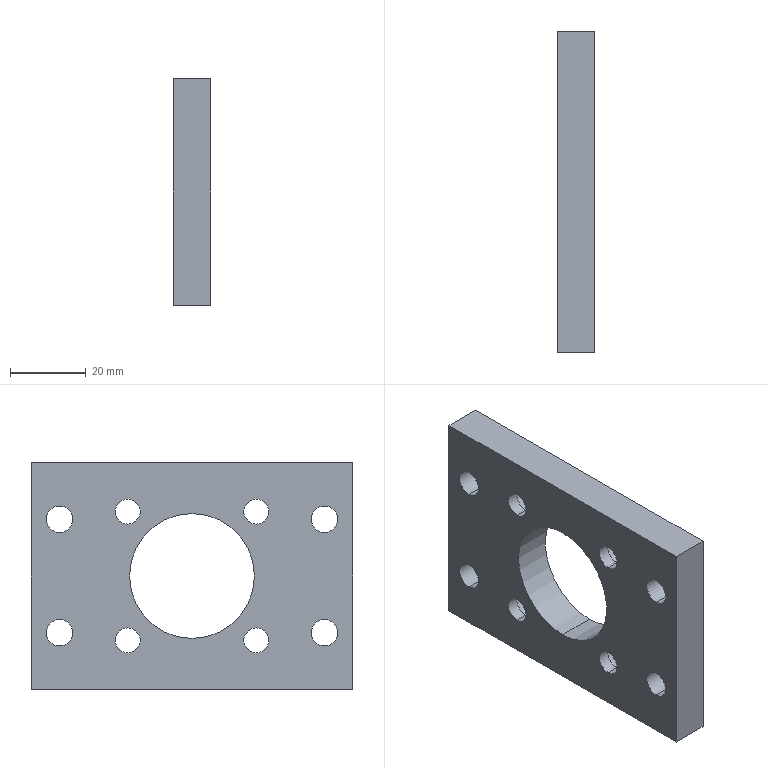Part | SolidWorks | features HoleWzd 2, Extrusion 1, ICE 1 | 1 solid | 36 faces | box 10 x 85 x 60 mm | volume 37885 mm3 | cylinder 26 | plane 10 | commonest cylinder face diameters 6.6 x8 7 x8 11 x8 33 x2
STEP:
#1=CARTESIAN_POINT('',(10.,0.,-16.5));
#2=VERTEX_POINT('',#1);
#3=CARTESIAN_POINT('',(10.,0.,16.5));
#4=VERTEX_POINT('',#3);
#5=CARTESIAN_POINT('',(10.,0.,0.));
#6=DIRECTION('',(-1.,0.,0.));
#7=DIRECTION('',(0.,0.,1.));
#8=AXIS2_PLACEMENT_3D('',#5,#6,#7);
#9=CIRCLE('',#8,16.5);
#10=EDGE_CURVE('',#2,#4,#9,.T.);
#11=ORIENTED_EDGE('',*,*,#10,.F.);
#12=CARTESIAN_POINT('',(0.,0.,-16.5));
#13=VERTEX_POINT('',#12);
#14=CARTESIAN_POINT('',(10.,0.,-16.5));
#15=DIRECTION('',(-1.,0.,0.));
#16=VECTOR('',#15,1000.);
#17=LINE('',#14,#16);
#18=EDGE_CURVE('',#2,#13,#17,.T.);
#19=ORIENTED_EDGE('',*,*,#18,.T.);
#20=CARTESIAN_POINT('',(0.,0.,16.5));
#21=VERTEX_POINT('',#20);
#22=CARTESIAN_POINT('',(0.,0.,0.));
#23=DIRECTION('',(-1.,0.,0.));
#24=DIRECTION('',(0.,0.,1.));
#25=AXIS2_PLACEMENT_3D('',#22,#23,#24);
#26=CIRCLE('',#25,16.5);
#27=EDGE_CURVE('',#13,#21,#26,.T.);
#28=ORIENTED_EDGE('',*,*,#27,.T.);
#29=CARTESIAN_POINT('',(10.,0.,16.5));
#30=DIRECTION('',(-1.,0.,0.));
#31=VECTOR('',#30,1000.);
#32=LINE('',#29,#31);
#33=EDGE_CURVE('',#4,#21,#32,.T.);
#34=ORIENTED_EDGE('',*,*,#33,.F.);
#35=EDGE_LOOP('',(#11,#19,#28,#34));
#36=FACE_OUTER_BOUND('',#35,.T.);
#37=CARTESIAN_POINT('',(10.,0.,0.));
#38=DIRECTION('',(-1.,0.,0.));
#39=DIRECTION('',(0.,0.,1.));
#40=AXIS2_PLACEMENT_3D('',#37,#38,#39);
#41=CYLINDRICAL_SURFACE('',#40,16.5);
#42=ADVANCED_FACE('',(#36),#41,.F.);
#43=CARTESIAN_POINT('',(10.,35.,-18.5));
#44=VERTEX_POINT('',#43);
#45=CARTESIAN_POINT('',(10.,35.,-11.5));
#46=VERTEX_POINT('',#45);
#47=CARTESIAN_POINT('',(10.,35.,-15.));
#48=DIRECTION('',(-1.,0.,0.));
#49=DIRECTION('',(0.,0.,1.));
#50=AXIS2_PLACEMENT_3D('',#47,#48,#49);
#51=CIRCLE('',#50,3.5);
#52=EDGE_CURVE('',#44,#46,#51,.T.);
#53=ORIENTED_EDGE('',*,*,#52,.F.);
#54=CARTESIAN_POINT('',(0.,35.,-18.5));
#55=VERTEX_POINT('',#54);
#56=CARTESIAN_POINT('',(0.,35.,-18.5));
#57=DIRECTION('',(-1.,0.,0.));
#58=VECTOR('',#57,1000.);
#59=LINE('',#56,#58);
#60=EDGE_CURVE('',#44,#55,#59,.T.);
#61=ORIENTED_EDGE('',*,*,#60,.T.);
#62=CARTESIAN_POINT('',(0.,35.,-11.5));
#63=VERTEX_POINT('',#62);
#64=CARTESIAN_POINT('',(0.,35.,-15.));
#65=DIRECTION('',(-1.,0.,0.));
#66=DIRECTION('',(0.,0.,1.));
#67=AXIS2_PLACEMENT_3D('',#64,#65,#66);
#68=CIRCLE('',#67,3.5);
#69=EDGE_CURVE('',#55,#63,#68,.T.);
#70=ORIENTED_EDGE('',*,*,#69,.T.);
#71=CARTESIAN_POINT('',(0.,35.,-11.5));
#72=DIRECTION('',(-1.,0.,0.));
#73=VECTOR('',#72,1000.);
#74=LINE('',#71,#73);
#75=EDGE_CURVE('',#46,#63,#74,.T.);
#76=ORIENTED_EDGE('',*,*,#75,.F.);
#77=EDGE_LOOP('',(#53,#61,#70,#76));
#78=FACE_OUTER_BOUND('',#77,.T.);
#79=CARTESIAN_POINT('',(0.,35.,-15.));
#80=DIRECTION('',(-1.,0.,0.));
#81=DIRECTION('',(0.,0.,1.));
#82=AXIS2_PLACEMENT_3D('',#79,#80,#81);
#83=CYLINDRICAL_SURFACE('',#82,3.5);
#84=ADVANCED_FACE('',(#78),#83,.F.);
#85=CARTESIAN_POINT('',(10.,35.,11.5));
#86=VERTEX_POINT('',#85);
#87=CARTESIAN_POINT('',(10.,35.,18.5));
#88=VERTEX_POINT('',#87);
#89=CARTESIAN_POINT('',(10.,35.,15.));
#90=DIRECTION('',(-1.,0.,0.));
#91=DIRECTION('',(0.,0.,1.));
#92=AXIS2_PLACEMENT_3D('',#89,#90,#91);
#93=CIRCLE('',#92,3.5);
#94=EDGE_CURVE('',#86,#88,#93,.T.);
#95=ORIENTED_EDGE('',*,*,#94,.F.);
#96=CARTESIAN_POINT('',(0.,35.,11.5));
#97=VERTEX_POINT('',#96);
#98=CARTESIAN_POINT('',(0.,35.,11.5));
#99=DIRECTION('',(-1.,0.,0.));
#100=VECTOR('',#99,1000.);
#101=LINE('',#98,#100);
#102=EDGE_CURVE('',#86,#97,#101,.T.);
#103=ORIENTED_EDGE('',*,*,#102,.T.);
#104=CARTESIAN_POINT('',(0.,35.,18.5));
#105=VERTEX_POINT('',#104);
#106=CARTESIAN_POINT('',(0.,35.,15.));
#107=DIRECTION('',(-1.,0.,0.));
#108=DIRECTION('',(0.,0.,1.));
#109=AXIS2_PLACEMENT_3D('',#106,#107,#108);
#110=CIRCLE('',#109,3.5);
#111=EDGE_CURVE('',#97,#105,#110,.T.);
#112=ORIENTED_EDGE('',*,*,#111,.T.);
#113=CARTESIAN_POINT('',(0.,35.,18.5));
#114=DIRECTION('',(-1.,0.,0.));
#115=VECTOR('',#114,1000.);
#116=LINE('',#113,#115);
#117=EDGE_CURVE('',#88,#105,#116,.T.);
#118=ORIENTED_EDGE('',*,*,#117,.F.);
#119=EDGE_LOOP('',(#95,#103,#112,#118));
#120=FACE_OUTER_BOUND('',#119,.T.);
#121=CARTESIAN_POINT('',(0.,35.,15.));
#122=DIRECTION('',(-1.,0.,0.));
#123=DIRECTION('',(0.,0.,1.));
#124=AXIS2_PLACEMENT_3D('',#121,#122,#123);
#125=CYLINDRICAL_SURFACE('',#124,3.5);
#126=ADVANCED_FACE('',(#120),#125,.F.);
#127=CARTESIAN_POINT('',(10.,-35.,-18.5));
#128=VERTEX_POINT('',#127);
#129=CARTESIAN_POINT('',(10.,-35.,-11.5));
#130=VERTEX_POINT('',#129);
#131=CARTESIAN_POINT('',(10.,-35.,-15.));
#132=DIRECTION('',(-1.,0.,0.));
#133=DIRECTION('',(0.,0.,1.));
#134=AXIS2_PLACEMENT_3D('',#131,#132,#133);
#135=CIRCLE('',#134,3.5);
#136=EDGE_CURVE('',#128,#130,#135,.T.);
#137=ORIENTED_EDGE('',*,*,#136,.F.);
#138=CARTESIAN_POINT('',(0.,-35.,-18.5));
#139=VERTEX_POINT('',#138);
#140=CARTESIAN_POINT('',(0.,-35.,-18.5));
#141=DIRECTION('',(-1.,0.,0.));
#142=VECTOR('',#141,1000.);
#143=LINE('',#140,#142);
#144=EDGE_CURVE('',#128,#139,#143,.T.);
#145=ORIENTED_EDGE('',*,*,#144,.T.);
#146=CARTESIAN_POINT('',(0.,-35.,-11.5));
#147=VERTEX_POINT('',#146);
#148=CARTESIAN_POINT('',(0.,-35.,-15.));
#149=DIRECTION('',(-1.,0.,0.));
#150=DIRECTION('',(0.,0.,1.));
#151=AXIS2_PLACEMENT_3D('',#148,#149,#150);
#152=CIRCLE('',#151,3.5);
#153=EDGE_CURVE('',#139,#147,#152,.T.);
#154=ORIENTED_EDGE('',*,*,#153,.T.);
#155=CARTESIAN_POINT('',(0.,-35.,-11.5));
#156=DIRECTION('',(-1.,0.,0.));
#157=VECTOR('',#156,1000.);
#158=LINE('',#155,#157);
#159=EDGE_CURVE('',#130,#147,#158,.T.);
#160=ORIENTED_EDGE('',*,*,#159,.F.);
#161=EDGE_LOOP('',(#137,#145,#154,#160));
#162=FACE_OUTER_BOUND('',#161,.T.);
#163=CARTESIAN_POINT('',(0.,-35.,-15.));
#164=DIRECTION('',(-1.,0.,0.));
#165=DIRECTION('',(0.,0.,1.));
#166=AXIS2_PLACEMENT_3D('',#163,#164,#165);
#167=CYLINDRICAL_SURFACE('',#166,3.5);
#168=ADVANCED_FACE('',(#162),#167,.F.);
#169=CARTESIAN_POINT('',(10.,-35.,11.5));
#170=VERTEX_POINT('',#169);
#171=CARTESIAN_POINT('',(10.,-35.,18.5));
#172=VERTEX_POINT('',#171);
#173=CARTESIAN_POINT('',(10.,-35.,15.));
#174=DIRECTION('',(-1.,0.,0.));
#175=DIRECTION('',(0.,0.,1.));
#176=AXIS2_PLACEMENT_3D('',#173,#174,#175);
#177=CIRCLE('',#176,3.5);
#178=EDGE_CURVE('',#170,#172,#177,.T.);
#179=ORIENTED_EDGE('',*,*,#178,.F.);
#180=CARTESIAN_POINT('',(0.,-35.,11.5));
#181=VERTEX_POINT('',#180);
#182=CARTESIAN_POINT('',(0.,-35.,11.5));
#183=DIRECTION('',(-1.,0.,0.));
#184=VECTOR('',#183,1000.);
#185=LINE('',#182,#184);
#186=EDGE_CURVE('',#170,#181,#185,.T.);
#187=ORIENTED_EDGE('',*,*,#186,.T.);
#188=CARTESIAN_POINT('',(0.,-35.,18.5));
#189=VERTEX_POINT('',#188);
#190=CARTESIAN_POINT('',(0.,-35.,15.));
#191=DIRECTION('',(-1.,0.,0.));
#192=DIRECTION('',(0.,0.,1.));
#193=AXIS2_PLACEMENT_3D('',#190,#191,#192);
#194=CIRCLE('',#193,3.5);
#195=EDGE_CURVE('',#181,#189,#194,.T.);
#196=ORIENTED_EDGE('',*,*,#195,.T.);
#197=CARTESIAN_POINT('',(0.,-35.,18.5));
#198=DIRECTION('',(-1.,0.,0.));
#199=VECTOR('',#198,1000.);
#200=LINE('',#197,#199);
#201=EDGE_CURVE('',#172,#189,#200,.T.);
#202=ORIENTED_EDGE('',*,*,#201,.F.);
#203=EDGE_LOOP('',(#179,#187,#196,#202));
#204=FACE_OUTER_BOUND('',#203,.T.);
#205=CARTESIAN_POINT('',(0.,-35.,15.));
#206=DIRECTION('',(-1.,0.,0.));
#207=DIRECTION('',(0.,0.,1.));
#208=AXIS2_PLACEMENT_3D('',#205,#206,#207);
#209=CYLINDRICAL_SURFACE('',#208,3.5);
#210=ADVANCED_FACE('',(#204),#209,.F.);
#211=CARTESIAN_POINT('',(3.2,17.,22.5));
#212=VERTEX_POINT('',#211);
#213=CARTESIAN_POINT('',(3.2,17.,11.5));
#214=VERTEX_POINT('',#213);
#215=CARTESIAN_POINT('',(3.2,17.,17.));
#216=DIRECTION('',(1.,0.,0.));
#217=DIRECTION('',(0.,0.,-1.));
#218=AXIS2_PLACEMENT_3D('',#215,#216,#217);
#219=CIRCLE('',#218,5.5);
#220=EDGE_CURVE('',#212,#214,#219,.T.);
#221=ORIENTED_EDGE('',*,*,#220,.F.);
#222=CARTESIAN_POINT('',(10.,17.,22.5));
#223=VERTEX_POINT('',#222);
#224=CARTESIAN_POINT('',(10.,17.,22.5));
#225=DIRECTION('',(1.,0.,0.));
#226=VECTOR('',#225,1000.);
#227=LINE('',#224,#226);
#228=EDGE_CURVE('',#212,#223,#227,.T.);
#229=ORIENTED_EDGE('',*,*,#228,.T.);
#230=CARTESIAN_POINT('',(10.,17.,11.5));
#231=VERTEX_POINT('',#230);
#232=CARTESIAN_POINT('',(10.,17.,17.));
#233=DIRECTION('',(1.,0.,0.));
#234=DIRECTION('',(0.,0.,-1.));
#235=AXIS2_PLACEMENT_3D('',#232,#233,#234);
#236=CIRCLE('',#235,5.5);
#237=EDGE_CURVE('',#223,#231,#236,.T.);
#238=ORIENTED_EDGE('',*,*,#237,.T.);
#239=CARTESIAN_POINT('',(10.,17.,11.5));
#240=DIRECTION('',(1.,0.,0.));
#241=VECTOR('',#240,1000.);
#242=LINE('',#239,#241);
#243=EDGE_CURVE('',#214,#231,#242,.T.);
#244=ORIENTED_EDGE('',*,*,#243,.F.);
#245=EDGE_LOOP('',(#221,#229,#238,#244));
#246=FACE_OUTER_BOUND('',#245,.T.);
#247=CARTESIAN_POINT('',(10.,17.,17.));
#248=DIRECTION('',(1.,0.,0.));
#249=DIRECTION('',(0.,0.,-1.));
#250=AXIS2_PLACEMENT_3D('',#247,#248,#249);
#251=CYLINDRICAL_SURFACE('',#250,5.5);
#252=ADVANCED_FACE('',(#246),#251,.F.);
#253=CARTESIAN_POINT('',(0.,17.,20.3));
#254=VERTEX_POINT('',#253);
#255=CARTESIAN_POINT('',(0.,17.,13.7));
#256=VERTEX_POINT('',#255);
#257=CARTESIAN_POINT('',(0.,17.,17.));
#258=DIRECTION('',(1.,0.,0.));
#259=DIRECTION('',(0.,0.,-1.));
#260=AXIS2_PLACEMENT_3D('',#257,#258,#259);
#261=CIRCLE('',#260,3.3);
#262=EDGE_CURVE('',#254,#256,#261,.T.);
#263=ORIENTED_EDGE('',*,*,#262,.F.);
#264=CARTESIAN_POINT('',(3.2,17.,20.3));
#265=VERTEX_POINT('',#264);
#266=CARTESIAN_POINT('',(10.,17.,20.3));
#267=DIRECTION('',(1.,0.,0.));
#268=VECTOR('',#267,1000.);
#269=LINE('',#266,#268);
#270=EDGE_CURVE('',#254,#265,#269,.T.);
#271=ORIENTED_EDGE('',*,*,#270,.T.);
#272=CARTESIAN_POINT('',(3.2,17.,13.7));
#273=VERTEX_POINT('',#272);
#274=CARTESIAN_POINT('',(3.2,17.,17.));
#275=DIRECTION('',(1.,0.,0.));
#276=DIRECTION('',(0.,0.,-1.));
#277=AXIS2_PLACEMENT_3D('',#274,#275,#276);
#278=CIRCLE('',#277,3.3);
#279=EDGE_CURVE('',#265,#273,#278,.T.);
#280=ORIENTED_EDGE('',*,*,#279,.T.);
#281=CARTESIAN_POINT('',(10.,17.,13.7));
#282=DIRECTION('',(1.,0.,0.));
#283=VECTOR('',#282,1000.);
#284=LINE('',#281,#283);
#285=EDGE_CURVE('',#256,#273,#284,.T.);
#286=ORIENTED_EDGE('',*,*,#285,.F.);
#287=EDGE_LOOP('',(#263,#271,#280,#286));
#288=FACE_OUTER_BOUND('',#287,.T.);
#289=CARTESIAN_POINT('',(10.,17.,17.));
#290=DIRECTION('',(1.,0.,0.));
#291=DIRECTION('',(0.,0.,-1.));
#292=AXIS2_PLACEMENT_3D('',#289,#290,#291);
#293=CYLINDRICAL_SURFACE('',#292,3.3);
#294=ADVANCED_FACE('',(#288),#293,.F.);
#295=CARTESIAN_POINT('',(3.2,17.,-11.5));
#296=VERTEX_POINT('',#295);
#297=CARTESIAN_POINT('',(3.2,17.,-22.5));
#298=VERTEX_POINT('',#297);
#299=CARTESIAN_POINT('',(3.2,17.,-17.));
#300=DIRECTION('',(1.,0.,0.));
#301=DIRECTION('',(0.,0.,-1.));
#302=AXIS2_PLACEMENT_3D('',#299,#300,#301);
#303=CIRCLE('',#302,5.5);
#304=EDGE_CURVE('',#296,#298,#303,.T.);
#305=ORIENTED_EDGE('',*,*,#304,.F.);
#306=CARTESIAN_POINT('',(10.,17.,-11.5));
#307=VERTEX_POINT('',#306);
#308=CARTESIAN_POINT('',(10.,17.,-11.5));
#309=DIRECTION('',(1.,0.,0.));
#310=VECTOR('',#309,1000.);
#311=LINE('',#308,#310);
#312=EDGE_CURVE('',#296,#307,#311,.T.);
#313=ORIENTED_EDGE('',*,*,#312,.T.);
#314=CARTESIAN_POINT('',(10.,17.,-22.5));
#315=VERTEX_POINT('',#314);
#316=CARTESIAN_POINT('',(10.,17.,-17.));
#317=DIRECTION('',(1.,0.,0.));
#318=DIRECTION('',(0.,0.,-1.));
#319=AXIS2_PLACEMENT_3D('',#316,#317,#318);
#320=CIRCLE('',#319,5.5);
#321=EDGE_CURVE('',#307,#315,#320,.T.);
#322=ORIENTED_EDGE('',*,*,#321,.T.);
#323=CARTESIAN_POINT('',(10.,17.,-22.5));
#324=DIRECTION('',(1.,0.,0.));
#325=VECTOR('',#324,1000.);
#326=LINE('',#323,#325);
#327=EDGE_CURVE('',#298,#315,#326,.T.);
#328=ORIENTED_EDGE('',*,*,#327,.F.);
#329=EDGE_LOOP('',(#305,#313,#322,#328));
#330=FACE_OUTER_BOUND('',#329,.T.);
#331=CARTESIAN_POINT('',(10.,17.,-17.));
#332=DIRECTION('',(1.,0.,0.));
#333=DIRECTION('',(0.,0.,-1.));
#334=AXIS2_PLACEMENT_3D('',#331,#332,#333);
#335=CYLINDRICAL_SURFACE('',#334,5.5);
#336=ADVANCED_FACE('',(#330),#335,.F.);
#337=CARTESIAN_POINT('',(0.,17.,-13.7));
#338=VERTEX_POINT('',#337);
#339=CARTESIAN_POINT('',(0.,17.,-20.3));
#340=VERTEX_POINT('',#339);
#341=CARTESIAN_POINT('',(0.,17.,-17.));
#342=DIRECTION('',(1.,0.,0.));
#343=DIRECTION('',(0.,0.,-1.));
#344=AXIS2_PLACEMENT_3D('',#341,#342,#343);
#345=CIRCLE('',#344,3.3);
#346=EDGE_CURVE('',#338,#340,#345,.T.);
#347=ORIENTED_EDGE('',*,*,#346,.F.);
#348=CARTESIAN_POINT('',(3.2,17.,-13.7));
#349=VERTEX_POINT('',#348);
#350=CARTESIAN_POINT('',(10.,17.,-13.7));
#351=DIRECTION('',(1.,0.,0.));
#352=VECTOR('',#351,1000.);
#353=LINE('',#350,#352);
#354=EDGE_CURVE('',#338,#349,#353,.T.);
#355=ORIENTED_EDGE('',*,*,#354,.T.);
#356=CARTESIAN_POINT('',(3.2,17.,-20.3));
#357=VERTEX_POINT('',#356);
#358=CARTESIAN_POINT('',(3.2,17.,-17.));
#359=DIRECTION('',(1.,0.,0.));
#360=DIRECTION('',(0.,0.,-1.));
#361=AXIS2_PLACEMENT_3D('',#358,#359,#360);
#362=CIRCLE('',#361,3.3);
#363=EDGE_CURVE('',#349,#357,#362,.T.);
#364=ORIENTED_EDGE('',*,*,#363,.T.);
#365=CARTESIAN_POINT('',(10.,17.,-20.3));
#366=DIRECTION('',(1.,0.,0.));
#367=VECTOR('',#366,1000.);
#368=LINE('',#365,#367);
#369=EDGE_CURVE('',#340,#357,#368,.T.);
#370=ORIENTED_EDGE('',*,*,#369,.F.);
#371=EDGE_LOOP('',(#347,#355,#364,#370));
#372=FACE_OUTER_BOUND('',#371,.T.);
#373=CARTESIAN_POINT('',(10.,17.,-17.));
#374=DIRECTION('',(1.,0.,0.));
#375=DIRECTION('',(0.,0.,-1.));
#376=AXIS2_PLACEMENT_3D('',#373,#374,#375);
#377=CYLINDRICAL_SURFACE('',#376,3.3);
#378=ADVANCED_FACE('',(#372),#377,.F.);
#379=CARTESIAN_POINT('',(3.2,-17.,22.5));
#380=VERTEX_POINT('',#379);
#381=CARTESIAN_POINT('',(3.2,-17.,11.5));
#382=VERTEX_POINT('',#381);
#383=CARTESIAN_POINT('',(3.2,-17.,17.));
#384=DIRECTION('',(1.,0.,0.));
#385=DIRECTION('',(0.,0.,-1.));
#386=AXIS2_PLACEMENT_3D('',#383,#384,#385);
#387=CIRCLE('',#386,5.5);
#388=EDGE_CURVE('',#380,#382,#387,.T.);
#389=ORIENTED_EDGE('',*,*,#388,.F.);
#390=CARTESIAN_POINT('',(10.,-17.,22.5));
#391=VERTEX_POINT('',#390);
#392=CARTESIAN_POINT('',(10.,-17.,22.5));
#393=DIRECTION('',(1.,0.,0.));
#394=VECTOR('',#393,1000.);
#395=LINE('',#392,#394);
#396=EDGE_CURVE('',#380,#391,#395,.T.);
#397=ORIENTED_EDGE('',*,*,#396,.T.);
#398=CARTESIAN_POINT('',(10.,-17.,11.5));
#399=VERTEX_POINT('',#398);
#400=CARTESIAN_POINT('',(10.,-17.,17.));
#401=DIRECTION('',(1.,0.,0.));
#402=DIRECTION('',(0.,0.,-1.));
#403=AXIS2_PLACEMENT_3D('',#400,#401,#402);
#404=CIRCLE('',#403,5.5);
#405=EDGE_CURVE('',#391,#399,#404,.T.);
#406=ORIENTED_EDGE('',*,*,#405,.T.);
#407=CARTESIAN_POINT('',(10.,-17.,11.5));
#408=DIRECTION('',(1.,0.,0.));
#409=VECTOR('',#408,1000.);
#410=LINE('',#407,#409);
#411=EDGE_CURVE('',#382,#399,#410,.T.);
#412=ORIENTED_EDGE('',*,*,#411,.F.);
#413=EDGE_LOOP('',(#389,#397,#406,#412));
#414=FACE_OUTER_BOUND('',#413,.T.);
#415=CARTESIAN_POINT('',(10.,-17.,17.));
#416=DIRECTION('',(1.,0.,0.));
#417=DIRECTION('',(0.,0.,-1.));
#418=AXIS2_PLACEMENT_3D('',#415,#416,#417);
#419=CYLINDRICAL_SURFACE('',#418,5.5);
#420=ADVANCED_FACE('',(#414),#419,.F.);
#421=CARTESIAN_POINT('',(0.,-17.,20.3));
#422=VERTEX_POINT('',#421);
#423=CARTESIAN_POINT('',(0.,-17.,13.7));
#424=VERTEX_POINT('',#423);
#425=CARTESIAN_POINT('',(0.,-17.,17.));
#426=DIRECTION('',(1.,0.,0.));
#427=DIRECTION('',(0.,0.,-1.));
#428=AXIS2_PLACEMENT_3D('',#425,#426,#427);
#429=CIRCLE('',#428,3.3);
#430=EDGE_CURVE('',#422,#424,#429,.T.);
#431=ORIENTED_EDGE('',*,*,#430,.F.);
#432=CARTESIAN_POINT('',(3.2,-17.,20.3));
#433=VERTEX_POINT('',#432);
#434=CARTESIAN_POINT('',(10.,-17.,20.3));
#435=DIRECTION('',(1.,0.,0.));
#436=VECTOR('',#435,1000.);
#437=LINE('',#434,#436);
#438=EDGE_CURVE('',#422,#433,#437,.T.);
#439=ORIENTED_EDGE('',*,*,#438,.T.);
#440=CARTESIAN_POINT('',(3.2,-17.,13.7));
#441=VERTEX_POINT('',#440);
#442=CARTESIAN_POINT('',(3.2,-17.,17.));
#443=DIRECTION('',(1.,0.,0.));
#444=DIRECTION('',(0.,0.,-1.));
#445=AXIS2_PLACEMENT_3D('',#442,#443,#444);
#446=CIRCLE('',#445,3.3);
#447=EDGE_CURVE('',#433,#441,#446,.T.);
#448=ORIENTED_EDGE('',*,*,#447,.T.);
#449=CARTESIAN_POINT('',(10.,-17.,13.7));
#450=DIRECTION('',(1.,0.,0.));
#451=VECTOR('',#450,1000.);
#452=LINE('',#449,#451);
#453=EDGE_CURVE('',#424,#441,#452,.T.);
#454=ORIENTED_EDGE('',*,*,#453,.F.);
#455=EDGE_LOOP('',(#431,#439,#448,#454));
#456=FACE_OUTER_BOUND('',#455,.T.);
#457=CARTESIAN_POINT('',(10.,-17.,17.));
#458=DIRECTION('',(1.,0.,0.));
#459=DIRECTION('',(0.,0.,-1.));
#460=AXIS2_PLACEMENT_3D('',#457,#458,#459);
#461=CYLINDRICAL_SURFACE('',#460,3.3);
#462=ADVANCED_FACE('',(#456),#461,.F.);
#463=CARTESIAN_POINT('',(3.2,-17.,-11.5));
#464=VERTEX_POINT('',#463);
#465=CARTESIAN_POINT('',(3.2,-17.,-22.5));
#466=VERTEX_POINT('',#465);
#467=CARTESIAN_POINT('',(3.2,-17.,-17.));
#468=DIRECTION('',(1.,0.,0.));
#469=DIRECTION('',(0.,0.,-1.));
#470=AXIS2_PLACEMENT_3D('',#467,#468,#469);
#471=CIRCLE('',#470,5.5);
#472=EDGE_CURVE('',#464,#466,#471,.T.);
#473=ORIENTED_EDGE('',*,*,#472,.F.);
#474=CARTESIAN_POINT('',(10.,-17.,-11.5));
#475=VERTEX_POINT('',#474);
#476=CARTESIAN_POINT('',(10.,-17.,-11.5));
#477=DIRECTION('',(1.,0.,0.));
#478=VECTOR('',#477,1000.);
#479=LINE('',#476,#478);
#480=EDGE_CURVE('',#464,#475,#479,.T.);
#481=ORIENTED_EDGE('',*,*,#480,.T.);
#482=CARTESIAN_POINT('',(10.,-17.,-22.5));
#483=VERTEX_POINT('',#482);
#484=CARTESIAN_POINT('',(10.,-17.,-17.));
#485=DIRECTION('',(1.,0.,0.));
#486=DIRECTION('',(0.,0.,-1.));
#487=AXIS2_PLACEMENT_3D('',#484,#485,#486);
#488=CIRCLE('',#487,5.5);
#489=EDGE_CURVE('',#475,#483,#488,.T.);
#490=ORIENTED_EDGE('',*,*,#489,.T.);
#491=CARTESIAN_POINT('',(10.,-17.,-22.5));
#492=DIRECTION('',(1.,0.,0.));
#493=VECTOR('',#492,1000.);
#494=LINE('',#491,#493);
#495=EDGE_CURVE('',#466,#483,#494,.T.);
#496=ORIENTED_EDGE('',*,*,#495,.F.);
#497=EDGE_LOOP('',(#473,#481,#490,#496));
#498=FACE_OUTER_BOUND('',#497,.T.);
#499=CARTESIAN_POINT('',(10.,-17.,-17.));
#500=DIRECTION('',(1.,0.,0.));
#501=DIRECTION('',(0.,0.,-1.));
#502=AXIS2_PLACEMENT_3D('',#499,#500,#501);
#503=CYLINDRICAL_SURFACE('',#502,5.5);
#504=ADVANCED_FACE('',(#498),#503,.F.);
#505=CARTESIAN_POINT('',(0.,-17.,-13.7));
#506=VERTEX_POINT('',#505);
#507=CARTESIAN_POINT('',(0.,-17.,-20.3));
#508=VERTEX_POINT('',#507);
#509=CARTESIAN_POINT('',(0.,-17.,-17.));
#510=DIRECTION('',(1.,0.,0.));
#511=DIRECTION('',(0.,0.,-1.));
#512=AXIS2_PLACEMENT_3D('',#509,#510,#511);
#513=CIRCLE('',#512,3.3);
#514=EDGE_CURVE('',#506,#508,#513,.T.);
#515=ORIENTED_EDGE('',*,*,#514,.F.);
#516=CARTESIAN_POINT('',(3.2,-17.,-13.7));
#517=VERTEX_POINT('',#516);
#518=CARTESIAN_POINT('',(10.,-17.,-13.7));
#519=DIRECTION('',(1.,0.,0.));
#520=VECTOR('',#519,1000.);
#521=LINE('',#518,#520);
#522=EDGE_CURVE('',#506,#517,#521,.T.);
#523=ORIENTED_EDGE('',*,*,#522,.T.);
#524=CARTESIAN_POINT('',(3.2,-17.,-20.3));
#525=VERTEX_POINT('',#524);
#526=CARTESIAN_POINT('',(3.2,-17.,-17.));
#527=DIRECTION('',(1.,0.,0.));
#528=DIRECTION('',(0.,0.,-1.));
#529=AXIS2_PLACEMENT_3D('',#526,#527,#528);
#530=CIRCLE('',#529,3.3);
#531=EDGE_CURVE('',#517,#525,#530,.T.);
#532=ORIENTED_EDGE('',*,*,#531,.T.);
#533=CARTESIAN_POINT('',(10.,-17.,-20.3));
#534=DIRECTION('',(1.,0.,0.));
#535=VECTOR('',#534,1000.);
#536=LINE('',#533,#535);
#537=EDGE_CURVE('',#508,#525,#536,.T.);
#538=ORIENTED_EDGE('',*,*,#537,.F.);
#539=EDGE_LOOP('',(#515,#523,#532,#538));
#540=FACE_OUTER_BOUND('',#539,.T.);
#541=CARTESIAN_POINT('',(10.,-17.,-17.));
#542=DIRECTION('',(1.,0.,0.));
#543=DIRECTION('',(0.,0.,-1.));
#544=AXIS2_PLACEMENT_3D('',#541,#542,#543);
#545=CYLINDRICAL_SURFACE('',#544,3.3);
#546=ADVANCED_FACE('',(#540),#545,.F.);
#547=CARTESIAN_POINT('',(0.,0.,0.));
#548=DIRECTION('',(-1.,0.,0.));
#549=DIRECTION('',(0.,0.,1.));
#550=AXIS2_PLACEMENT_3D('',#547,#548,#549);
#551=CIRCLE('',#550,16.5);
#552=EDGE_CURVE('',#21,#13,#551,.T.);
#553=ORIENTED_EDGE('',*,*,#552,.F.);
#554=ORIENTED_EDGE('',*,*,#27,.F.);
#555=EDGE_LOOP('',(#553,#554));
#556=FACE_BOUND('',#555,.T.);
#557=CARTESIAN_POINT('',(0.,35.,-15.));
#558=DIRECTION('',(-1.,0.,0.));
#559=DIRECTION('',(0.,0.,1.));
#560=AXIS2_PLACEMENT_3D('',#557,#558,#559);
#561=CIRCLE('',#560,3.5);
#562=EDGE_CURVE('',#63,#55,#561,.T.);
#563=ORIENTED_EDGE('',*,*,#562,.F.);
#564=ORIENTED_EDGE('',*,*,#69,.F.);
#565=EDGE_LOOP('',(#563,#564));
#566=FACE_BOUND('',#565,.T.);
#567=CARTESIAN_POINT('',(0.,-35.,-15.));
#568=DIRECTION('',(-1.,0.,0.));
#569=DIRECTION('',(0.,0.,1.));
#570=AXIS2_PLACEMENT_3D('',#567,#568,#569);
#571=CIRCLE('',#570,3.5);
#572=EDGE_CURVE('',#147,#139,#571,.T.);
#573=ORIENTED_EDGE('',*,*,#572,.F.);
#574=ORIENTED_EDGE('',*,*,#153,.F.);
#575=EDGE_LOOP('',(#573,#574));
#576=FACE_BOUND('',#575,.T.);
#577=CARTESIAN_POINT('',(0.,-35.,15.));
#578=DIRECTION('',(-1.,0.,0.));
#579=DIRECTION('',(0.,0.,1.));
#580=AXIS2_PLACEMENT_3D('',#577,#578,#579);
#581=CIRCLE('',#580,3.5);
#582=EDGE_CURVE('',#189,#181,#581,.T.);
#583=ORIENTED_EDGE('',*,*,#582,.F.);
#584=ORIENTED_EDGE('',*,*,#195,.F.);
#585=EDGE_LOOP('',(#583,#584));
#586=FACE_BOUND('',#585,.T.);
#587=CARTESIAN_POINT('',(0.,17.,17.));
#588=DIRECTION('',(1.,0.,0.));
#589=DIRECTION('',(0.,0.,-1.));
#590=AXIS2_PLACEMENT_3D('',#587,#588,#589);
#591=CIRCLE('',#590,3.3);
#592=EDGE_CURVE('',#256,#254,#591,.T.);
#593=ORIENTED_EDGE('',*,*,#592,.T.);
#594=ORIENTED_EDGE('',*,*,#262,.T.);
#595=EDGE_LOOP('',(#593,#594));
#596=FACE_BOUND('',#595,.T.);
#597=CARTESIAN_POINT('',(0.,17.,-17.));
#598=DIRECTION('',(1.,0.,0.));
#599=DIRECTION('',(0.,0.,-1.));
#600=AXIS2_PLACEMENT_3D('',#597,#598,#599);
#601=CIRCLE('',#600,3.3);
#602=EDGE_CURVE('',#340,#338,#601,.T.);
#603=ORIENTED_EDGE('',*,*,#602,.T.);
#604=ORIENTED_EDGE('',*,*,#346,.T.);
#605=EDGE_LOOP('',(#603,#604));
#606=FACE_BOUND('',#605,.T.);
#607=CARTESIAN_POINT('',(0.,-17.,17.));
#608=DIRECTION('',(1.,0.,0.));
#609=DIRECTION('',(0.,0.,-1.));
#610=AXIS2_PLACEMENT_3D('',#607,#608,#609);
#611=CIRCLE('',#610,3.3);
#612=EDGE_CURVE('',#424,#422,#611,.T.);
#613=ORIENTED_EDGE('',*,*,#612,.T.);
#614=ORIENTED_EDGE('',*,*,#430,.T.);
#615=EDGE_LOOP('',(#613,#614));
#616=FACE_BOUND('',#615,.T.);
#617=CARTESIAN_POINT('',(0.,-17.,-17.));
#618=DIRECTION('',(1.,0.,0.));
#619=DIRECTION('',(0.,0.,-1.));
#620=AXIS2_PLACEMENT_3D('',#617,#618,#619);
#621=CIRCLE('',#620,3.3);
#622=EDGE_CURVE('',#508,#506,#621,.T.);
#623=ORIENTED_EDGE('',*,*,#622,.T.);
#624=ORIENTED_EDGE('',*,*,#514,.T.);
#625=EDGE_LOOP('',(#623,#624));
#626=FACE_BOUND('',#625,.T.);
#627=CARTESIAN_POINT('',(0.,-42.5,-30.));
#628=VERTEX_POINT('',#627);
#629=CARTESIAN_POINT('',(0.,42.5,-30.));
#630=VERTEX_POINT('',#629);
#631=CARTESIAN_POINT('',(0.,42.5,-30.));
#632=DIRECTION('',(0.,1.,0.));
#633=VECTOR('',#632,1000.);
#634=LINE('',#631,#633);
#635=EDGE_CURVE('',#628,#630,#634,.T.);
#636=ORIENTED_EDGE('',*,*,#635,.F.);
#637=CARTESIAN_POINT('',(0.,-42.5,30.));
#638=VERTEX_POINT('',#637);
#639=CARTESIAN_POINT('',(0.,-42.5,30.));
#640=DIRECTION('',(0.,0.,-1.));
#641=VECTOR('',#640,1000.);
#642=LINE('',#639,#641);
#643=EDGE_CURVE('',#638,#628,#642,.T.);
#644=ORIENTED_EDGE('',*,*,#643,.F.);
#645=CARTESIAN_POINT('',(0.,42.5,30.));
#646=VERTEX_POINT('',#645);
#647=CARTESIAN_POINT('',(0.,42.5,30.));
#648=DIRECTION('',(0.,-1.,0.));
#649=VECTOR('',#648,1000.);
#650=LINE('',#647,#649);
#651=EDGE_CURVE('',#646,#638,#650,.T.);
#652=ORIENTED_EDGE('',*,*,#651,.F.);
#653=CARTESIAN_POINT('',(0.,42.5,30.));
#654=DIRECTION('',(0.,0.,1.));
#655=VECTOR('',#654,1000.);
#656=LINE('',#653,#655);
#657=EDGE_CURVE('',#630,#646,#656,.T.);
#658=ORIENTED_EDGE('',*,*,#657,.F.);
#659=EDGE_LOOP('',(#636,#644,#652,#658));
#660=FACE_OUTER_BOUND('',#659,.T.);
#661=CARTESIAN_POINT('',(0.,35.,15.));
#662=DIRECTION('',(-1.,0.,0.));
#663=DIRECTION('',(0.,0.,1.));
#664=AXIS2_PLACEMENT_3D('',#661,#662,#663);
#665=CIRCLE('',#664,3.5);
#666=EDGE_CURVE('',#105,#97,#665,.T.);
#667=ORIENTED_EDGE('',*,*,#666,.F.);
#668=ORIENTED_EDGE('',*,*,#111,.F.);
#669=EDGE_LOOP('',(#667,#668));
#670=FACE_BOUND('',#669,.T.);
#671=CARTESIAN_POINT('',(0.,0.,0.));
#672=DIRECTION('',(1.,0.,0.));
#673=DIRECTION('',(0.,0.,-1.));
#674=AXIS2_PLACEMENT_3D('',#671,#672,#673);
#675=PLANE('',#674);
#676=ADVANCED_FACE('',(#556,#566,#576,#586,#596,#606,#616,#626,#660,#670),#675,.F.);
#677=ORIENTED_EDGE('',*,*,#635,.T.);
#678=CARTESIAN_POINT('',(10.,42.5,-30.));
#679=VERTEX_POINT('',#678);
#680=CARTESIAN_POINT('',(10.,42.5,-30.));
#681=DIRECTION('',(-1.,0.,0.));
#682=VECTOR('',#681,1000.);
#683=LINE('',#680,#682);
#684=EDGE_CURVE('',#679,#630,#683,.T.);
#685=ORIENTED_EDGE('',*,*,#684,.F.);
#686=CARTESIAN_POINT('',(10.,-42.5,-30.));
#687=VERTEX_POINT('',#686);
#688=CARTESIAN_POINT('',(10.,42.5,-30.));
#689=DIRECTION('',(0.,1.,0.));
#690=VECTOR('',#689,1000.);
#691=LINE('',#688,#690);
#692=EDGE_CURVE('',#687,#679,#691,.T.);
#693=ORIENTED_EDGE('',*,*,#692,.F.);
#694=CARTESIAN_POINT('',(10.,-42.5,-30.));
#695=DIRECTION('',(-1.,0.,0.));
#696=VECTOR('',#695,1000.);
#697=LINE('',#694,#696);
#698=EDGE_CURVE('',#687,#628,#697,.T.);
#699=ORIENTED_EDGE('',*,*,#698,.T.);
#700=EDGE_LOOP('',(#677,#685,#693,#699));
#701=FACE_OUTER_BOUND('',#700,.T.);
#702=CARTESIAN_POINT('',(10.,42.5,-30.));
#703=DIRECTION('',(0.,0.,1.));
#704=DIRECTION('',(0.,-1.,0.));
#705=AXIS2_PLACEMENT_3D('',#702,#703,#704);
#706=PLANE('',#705);
#707=ADVANCED_FACE('',(#701),#706,.F.);
#708=ORIENTED_EDGE('',*,*,#657,.T.);
#709=CARTESIAN_POINT('',(10.,42.5,30.));
#710=VERTEX_POINT('',#709);
#711=CARTESIAN_POINT('',(10.,42.5,30.));
#712=DIRECTION('',(-1.,0.,0.));
#713=VECTOR('',#712,1000.);
#714=LINE('',#711,#713);
#715=EDGE_CURVE('',#710,#646,#714,.T.);
#716=ORIENTED_EDGE('',*,*,#715,.F.);
#717=CARTESIAN_POINT('',(10.,42.5,30.));
#718=DIRECTION('',(0.,0.,1.));
#719=VECTOR('',#718,1000.);
#720=LINE('',#717,#719);
#721=EDGE_CURVE('',#679,#710,#720,.T.);
#722=ORIENTED_EDGE('',*,*,#721,.F.);
#723=ORIENTED_EDGE('',*,*,#684,.T.);
#724=EDGE_LOOP('',(#708,#716,#722,#723));
#725=FACE_OUTER_BOUND('',#724,.T.);
#726=CARTESIAN_POINT('',(10.,42.5,30.));
#727=DIRECTION('',(0.,-1.,0.));
#728=DIRECTION('',(0.,0.,-1.));
#729=AXIS2_PLACEMENT_3D('',#726,#727,#728);
#730=PLANE('',#729);
#731=ADVANCED_FACE('',(#725),#730,.F.);
#732=ORIENTED_EDGE('',*,*,#651,.T.);
#733=CARTESIAN_POINT('',(10.,-42.5,30.));
#734=VERTEX_POINT('',#733);
#735=CARTESIAN_POINT('',(10.,-42.5,30.));
#736=DIRECTION('',(-1.,0.,0.));
#737=VECTOR('',#736,1000.);
#738=LINE('',#735,#737);
#739=EDGE_CURVE('',#734,#638,#738,.T.);
#740=ORIENTED_EDGE('',*,*,#739,.F.);
#741=CARTESIAN_POINT('',(10.,42.5,30.));
#742=DIRECTION('',(0.,-1.,0.));
#743=VECTOR('',#742,1000.);
#744=LINE('',#741,#743);
#745=EDGE_CURVE('',#710,#734,#744,.T.);
#746=ORIENTED_EDGE('',*,*,#745,.F.);
#747=ORIENTED_EDGE('',*,*,#715,.T.);
#748=EDGE_LOOP('',(#732,#740,#746,#747));
#749=FACE_OUTER_BOUND('',#748,.T.);
#750=CARTESIAN_POINT('',(10.,42.5,30.));
#751=DIRECTION('',(0.,0.,-1.));
#752=DIRECTION('',(0.,1.,0.));
#753=AXIS2_PLACEMENT_3D('',#750,#751,#752);
#754=PLANE('',#753);
#755=ADVANCED_FACE('',(#749),#754,.F.);
#756=ORIENTED_EDGE('',*,*,#643,.T.);
#757=ORIENTED_EDGE('',*,*,#698,.F.);
#758=CARTESIAN_POINT('',(10.,-42.5,30.));
#759=DIRECTION('',(0.,0.,-1.));
#760=VECTOR('',#759,1000.);
#761=LINE('',#758,#760);
#762=EDGE_CURVE('',#734,#687,#761,.T.);
#763=ORIENTED_EDGE('',*,*,#762,.F.);
#764=ORIENTED_EDGE('',*,*,#739,.T.);
#765=EDGE_LOOP('',(#756,#757,#763,#764));
#766=FACE_OUTER_BOUND('',#765,.T.);
#767=CARTESIAN_POINT('',(10.,-42.5,30.));
#768=DIRECTION('',(0.,1.,0.));
#769=DIRECTION('',(0.,0.,1.));
#770=AXIS2_PLACEMENT_3D('',#767,#768,#769);
#771=PLANE('',#770);
#772=ADVANCED_FACE('',(#766),#771,.F.);
#773=CARTESIAN_POINT('',(10.,0.,0.));
#774=DIRECTION('',(-1.,0.,0.));
#775=DIRECTION('',(0.,0.,1.));
#776=AXIS2_PLACEMENT_3D('',#773,#774,#775);
#777=CIRCLE('',#776,16.5);
#778=EDGE_CURVE('',#4,#2,#777,.T.);
#779=ORIENTED_EDGE('',*,*,#778,.T.);
#780=ORIENTED_EDGE('',*,*,#10,.T.);
#781=EDGE_LOOP('',(#779,#780));
#782=FACE_BOUND('',#781,.T.);
#783=CARTESIAN_POINT('',(10.,35.,-15.));
#784=DIRECTION('',(-1.,0.,0.));
#785=DIRECTION('',(0.,0.,1.));
#786=AXIS2_PLACEMENT_3D('',#783,#784,#785);
#787=CIRCLE('',#786,3.5);
#788=EDGE_CURVE('',#46,#44,#787,.T.);
#789=ORIENTED_EDGE('',*,*,#788,.T.);
#790=ORIENTED_EDGE('',*,*,#52,.T.);
#791=EDGE_LOOP('',(#789,#790));
#792=FACE_BOUND('',#791,.T.);
#793=CARTESIAN_POINT('',(10.,35.,15.));
#794=DIRECTION('',(-1.,0.,0.));
#795=DIRECTION('',(0.,0.,1.));
#796=AXIS2_PLACEMENT_3D('',#793,#794,#795);
#797=CIRCLE('',#796,3.5);
#798=EDGE_CURVE('',#88,#86,#797,.T.);
#799=ORIENTED_EDGE('',*,*,#798,.T.);
#800=ORIENTED_EDGE('',*,*,#94,.T.);
#801=EDGE_LOOP('',(#799,#800));
#802=FACE_BOUND('',#801,.T.);
#803=CARTESIAN_POINT('',(10.,-35.,-15.));
#804=DIRECTION('',(-1.,0.,0.));
#805=DIRECTION('',(0.,0.,1.));
#806=AXIS2_PLACEMENT_3D('',#803,#804,#805);
#807=CIRCLE('',#806,3.5);
#808=EDGE_CURVE('',#130,#128,#807,.T.);
#809=ORIENTED_EDGE('',*,*,#808,.T.);
#810=ORIENTED_EDGE('',*,*,#136,.T.);
#811=EDGE_LOOP('',(#809,#810));
#812=FACE_BOUND('',#811,.T.);
#813=CARTESIAN_POINT('',(10.,-35.,15.));
#814=DIRECTION('',(-1.,0.,0.));
#815=DIRECTION('',(0.,0.,1.));
#816=AXIS2_PLACEMENT_3D('',#813,#814,#815);
#817=CIRCLE('',#816,3.5);
#818=EDGE_CURVE('',#172,#170,#817,.T.);
#819=ORIENTED_EDGE('',*,*,#818,.T.);
#820=ORIENTED_EDGE('',*,*,#178,.T.);
#821=EDGE_LOOP('',(#819,#820));
#822=FACE_BOUND('',#821,.T.);
#823=CARTESIAN_POINT('',(10.,17.,17.));
#824=DIRECTION('',(1.,0.,0.));
#825=DIRECTION('',(0.,0.,-1.));
#826=AXIS2_PLACEMENT_3D('',#823,#824,#825);
#827=CIRCLE('',#826,5.5);
#828=EDGE_CURVE('',#231,#223,#827,.T.);
#829=ORIENTED_EDGE('',*,*,#828,.F.);
#830=ORIENTED_EDGE('',*,*,#237,.F.);
#831=EDGE_LOOP('',(#829,#830));
#832=FACE_BOUND('',#831,.T.);
#833=CARTESIAN_POINT('',(10.,17.,-17.));
#834=DIRECTION('',(1.,0.,0.));
#835=DIRECTION('',(0.,0.,-1.));
#836=AXIS2_PLACEMENT_3D('',#833,#834,#835);
#837=CIRCLE('',#836,5.5);
#838=EDGE_CURVE('',#315,#307,#837,.T.);
#839=ORIENTED_EDGE('',*,*,#838,.F.);
#840=ORIENTED_EDGE('',*,*,#321,.F.);
#841=EDGE_LOOP('',(#839,#840));
#842=FACE_BOUND('',#841,.T.);
#843=CARTESIAN_POINT('',(10.,-17.,17.));
#844=DIRECTION('',(1.,0.,0.));
#845=DIRECTION('',(0.,0.,-1.));
#846=AXIS2_PLACEMENT_3D('',#843,#844,#845);
#847=CIRCLE('',#846,5.5);
#848=EDGE_CURVE('',#399,#391,#847,.T.);
#849=ORIENTED_EDGE('',*,*,#848,.F.);
#850=ORIENTED_EDGE('',*,*,#405,.F.);
#851=EDGE_LOOP('',(#849,#850));
#852=FACE_BOUND('',#851,.T.);
#853=CARTESIAN_POINT('',(10.,-17.,-17.));
#854=DIRECTION('',(1.,0.,0.));
#855=DIRECTION('',(0.,0.,-1.));
#856=AXIS2_PLACEMENT_3D('',#853,#854,#855);
#857=CIRCLE('',#856,5.5);
#858=EDGE_CURVE('',#483,#475,#857,.T.);
#859=ORIENTED_EDGE('',*,*,#858,.F.);
#860=ORIENTED_EDGE('',*,*,#489,.F.);
#861=EDGE_LOOP('',(#859,#860));
#862=FACE_BOUND('',#861,.T.);
#863=ORIENTED_EDGE('',*,*,#692,.T.);
#864=ORIENTED_EDGE('',*,*,#721,.T.);
#865=ORIENTED_EDGE('',*,*,#745,.T.);
#866=ORIENTED_EDGE('',*,*,#762,.T.);
#867=EDGE_LOOP('',(#863,#864,#865,#866));
#868=FACE_OUTER_BOUND('',#867,.T.);
#869=CARTESIAN_POINT('',(10.,0.,0.));
#870=DIRECTION('',(1.,0.,0.));
#871=DIRECTION('',(0.,0.,-1.));
#872=AXIS2_PLACEMENT_3D('',#869,#870,#871);
#873=PLANE('',#872);
#874=ADVANCED_FACE('',(#782,#792,#802,#812,#822,#832,#842,#852,#862,#868),#873,.T.);
#875=ORIENTED_EDGE('',*,*,#522,.F.);
#876=ORIENTED_EDGE('',*,*,#622,.F.);
#877=ORIENTED_EDGE('',*,*,#537,.T.);
#878=CARTESIAN_POINT('',(3.2,-17.,-17.));
#879=DIRECTION('',(1.,0.,0.));
#880=DIRECTION('',(0.,0.,-1.));
#881=AXIS2_PLACEMENT_3D('',#878,#879,#880);
#882=CIRCLE('',#881,3.3);
#883=EDGE_CURVE('',#525,#517,#882,.T.);
#884=ORIENTED_EDGE('',*,*,#883,.T.);
#885=EDGE_LOOP('',(#875,#876,#877,#884));
#886=FACE_OUTER_BOUND('',#885,.T.);
#887=CARTESIAN_POINT('',(10.,-17.,-17.));
#888=DIRECTION('',(1.,0.,0.));
#889=DIRECTION('',(0.,0.,-1.));
#890=AXIS2_PLACEMENT_3D('',#887,#888,#889);
#891=CYLINDRICAL_SURFACE('',#890,3.3);
#892=ADVANCED_FACE('',(#886),#891,.F.);
#893=ORIENTED_EDGE('',*,*,#883,.F.);
#894=ORIENTED_EDGE('',*,*,#531,.F.);
#895=EDGE_LOOP('',(#893,#894));
#896=FACE_BOUND('',#895,.T.);
#897=CARTESIAN_POINT('',(3.2,-17.,-17.));
#898=DIRECTION('',(1.,0.,0.));
#899=DIRECTION('',(0.,0.,-1.));
#900=AXIS2_PLACEMENT_3D('',#897,#898,#899);
#901=CIRCLE('',#900,5.5);
#902=EDGE_CURVE('',#466,#464,#901,.T.);
#903=ORIENTED_EDGE('',*,*,#902,.T.);
#904=ORIENTED_EDGE('',*,*,#472,.T.);
#905=EDGE_LOOP('',(#903,#904));
#906=FACE_OUTER_BOUND('',#905,.T.);
#907=CARTESIAN_POINT('',(3.2,-13.7,-17.));
#908=DIRECTION('',(-1.,0.,0.));
#909=DIRECTION('',(0.,0.,1.));
#910=AXIS2_PLACEMENT_3D('',#907,#908,#909);
#911=PLANE('',#910);
#912=ADVANCED_FACE('',(#896,#906),#911,.F.);
#913=ORIENTED_EDGE('',*,*,#480,.F.);
#914=ORIENTED_EDGE('',*,*,#902,.F.);
#915=ORIENTED_EDGE('',*,*,#495,.T.);
#916=ORIENTED_EDGE('',*,*,#858,.T.);
#917=EDGE_LOOP('',(#913,#914,#915,#916));
#918=FACE_OUTER_BOUND('',#917,.T.);
#919=CARTESIAN_POINT('',(10.,-17.,-17.));
#920=DIRECTION('',(1.,0.,0.));
#921=DIRECTION('',(0.,0.,-1.));
#922=AXIS2_PLACEMENT_3D('',#919,#920,#921);
#923=CYLINDRICAL_SURFACE('',#922,5.5);
#924=ADVANCED_FACE('',(#918),#923,.F.);
#925=ORIENTED_EDGE('',*,*,#438,.F.);
#926=ORIENTED_EDGE('',*,*,#612,.F.);
#927=ORIENTED_EDGE('',*,*,#453,.T.);
#928=CARTESIAN_POINT('',(3.2,-17.,17.));
#929=DIRECTION('',(1.,0.,0.));
#930=DIRECTION('',(0.,0.,-1.));
#931=AXIS2_PLACEMENT_3D('',#928,#929,#930);
#932=CIRCLE('',#931,3.3);
#933=EDGE_CURVE('',#441,#433,#932,.T.);
#934=ORIENTED_EDGE('',*,*,#933,.T.);
#935=EDGE_LOOP('',(#925,#926,#927,#934));
#936=FACE_OUTER_BOUND('',#935,.T.);
#937=CARTESIAN_POINT('',(10.,-17.,17.));
#938=DIRECTION('',(1.,0.,0.));
#939=DIRECTION('',(0.,0.,-1.));
#940=AXIS2_PLACEMENT_3D('',#937,#938,#939);
#941=CYLINDRICAL_SURFACE('',#940,3.3);
#942=ADVANCED_FACE('',(#936),#941,.F.);
#943=ORIENTED_EDGE('',*,*,#933,.F.);
#944=ORIENTED_EDGE('',*,*,#447,.F.);
#945=EDGE_LOOP('',(#943,#944));
#946=FACE_BOUND('',#945,.T.);
#947=CARTESIAN_POINT('',(3.2,-17.,17.));
#948=DIRECTION('',(1.,0.,0.));
#949=DIRECTION('',(0.,0.,-1.));
#950=AXIS2_PLACEMENT_3D('',#947,#948,#949);
#951=CIRCLE('',#950,5.5);
#952=EDGE_CURVE('',#382,#380,#951,.T.);
#953=ORIENTED_EDGE('',*,*,#952,.T.);
#954=ORIENTED_EDGE('',*,*,#388,.T.);
#955=EDGE_LOOP('',(#953,#954));
#956=FACE_OUTER_BOUND('',#955,.T.);
#957=CARTESIAN_POINT('',(3.2,-13.7,17.));
#958=DIRECTION('',(-1.,0.,0.));
#959=DIRECTION('',(0.,0.,1.));
#960=AXIS2_PLACEMENT_3D('',#957,#958,#959);
#961=PLANE('',#960);
#962=ADVANCED_FACE('',(#946,#956),#961,.F.);
#963=ORIENTED_EDGE('',*,*,#396,.F.);
#964=ORIENTED_EDGE('',*,*,#952,.F.);
#965=ORIENTED_EDGE('',*,*,#411,.T.);
#966=ORIENTED_EDGE('',*,*,#848,.T.);
#967=EDGE_LOOP('',(#963,#964,#965,#966));
#968=FACE_OUTER_BOUND('',#967,.T.);
#969=CARTESIAN_POINT('',(10.,-17.,17.));
#970=DIRECTION('',(1.,0.,0.));
#971=DIRECTION('',(0.,0.,-1.));
#972=AXIS2_PLACEMENT_3D('',#969,#970,#971);
#973=CYLINDRICAL_SURFACE('',#972,5.5);
#974=ADVANCED_FACE('',(#968),#973,.F.);
#975=ORIENTED_EDGE('',*,*,#354,.F.);
#976=ORIENTED_EDGE('',*,*,#602,.F.);
#977=ORIENTED_EDGE('',*,*,#369,.T.);
#978=CARTESIAN_POINT('',(3.2,17.,-17.));
#979=DIRECTION('',(1.,0.,0.));
#980=DIRECTION('',(0.,0.,-1.));
#981=AXIS2_PLACEMENT_3D('',#978,#979,#980);
#982=CIRCLE('',#981,3.3);
#983=EDGE_CURVE('',#357,#349,#982,.T.);
#984=ORIENTED_EDGE('',*,*,#983,.T.);
#985=EDGE_LOOP('',(#975,#976,#977,#984));
#986=FACE_OUTER_BOUND('',#985,.T.);
#987=CARTESIAN_POINT('',(10.,17.,-17.));
#988=DIRECTION('',(1.,0.,0.));
#989=DIRECTION('',(0.,0.,-1.));
#990=AXIS2_PLACEMENT_3D('',#987,#988,#989);
#991=CYLINDRICAL_SURFACE('',#990,3.3);
#992=ADVANCED_FACE('',(#986),#991,.F.);
#993=ORIENTED_EDGE('',*,*,#983,.F.);
#994=ORIENTED_EDGE('',*,*,#363,.F.);
#995=EDGE_LOOP('',(#993,#994));
#996=FACE_BOUND('',#995,.T.);
#997=CARTESIAN_POINT('',(3.2,17.,-17.));
#998=DIRECTION('',(1.,0.,0.));
#999=DIRECTION('',(0.,0.,-1.));
#1000=AXIS2_PLACEMENT_3D('',#997,#998,#999);
#1001=CIRCLE('',#1000,5.5);
#1002=EDGE_CURVE('',#298,#296,#1001,.T.);
#1003=ORIENTED_EDGE('',*,*,#1002,.T.);
#1004=ORIENTED_EDGE('',*,*,#304,.T.);
#1005=EDGE_LOOP('',(#1003,#1004));
#1006=FACE_OUTER_BOUND('',#1005,.T.);
#1007=CARTESIAN_POINT('',(3.2,20.3,-17.));
#1008=DIRECTION('',(-1.,0.,0.));
#1009=DIRECTION('',(0.,0.,1.));
#1010=AXIS2_PLACEMENT_3D('',#1007,#1008,#1009);
#1011=PLANE('',#1010);
#1012=ADVANCED_FACE('',(#996,#1006),#1011,.F.);
#1013=ORIENTED_EDGE('',*,*,#312,.F.);
#1014=ORIENTED_EDGE('',*,*,#1002,.F.);
#1015=ORIENTED_EDGE('',*,*,#327,.T.);
#1016=ORIENTED_EDGE('',*,*,#838,.T.);
#1017=EDGE_LOOP('',(#1013,#1014,#1015,#1016));
#1018=FACE_OUTER_BOUND('',#1017,.T.);
#1019=CARTESIAN_POINT('',(10.,17.,-17.));
#1020=DIRECTION('',(1.,0.,0.));
#1021=DIRECTION('',(0.,0.,-1.));
#1022=AXIS2_PLACEMENT_3D('',#1019,#1020,#1021);
#1023=CYLINDRICAL_SURFACE('',#1022,5.5);
#1024=ADVANCED_FACE('',(#1018),#1023,.F.);
#1025=ORIENTED_EDGE('',*,*,#270,.F.);
#1026=ORIENTED_EDGE('',*,*,#592,.F.);
#1027=ORIENTED_EDGE('',*,*,#285,.T.);
#1028=CARTESIAN_POINT('',(3.2,17.,17.));
#1029=DIRECTION('',(1.,0.,0.));
#1030=DIRECTION('',(0.,0.,-1.));
#1031=AXIS2_PLACEMENT_3D('',#1028,#1029,#1030);
#1032=CIRCLE('',#1031,3.3);
#1033=EDGE_CURVE('',#273,#265,#1032,.T.);
#1034=ORIENTED_EDGE('',*,*,#1033,.T.);
#1035=EDGE_LOOP('',(#1025,#1026,#1027,#1034));
#1036=FACE_OUTER_BOUND('',#1035,.T.);
#1037=CARTESIAN_POINT('',(10.,17.,17.));
#1038=DIRECTION('',(1.,0.,0.));
#1039=DIRECTION('',(0.,0.,-1.));
#1040=AXIS2_PLACEMENT_3D('',#1037,#1038,#1039);
#1041=CYLINDRICAL_SURFACE('',#1040,3.3);
#1042=ADVANCED_FACE('',(#1036),#1041,.F.);
#1043=ORIENTED_EDGE('',*,*,#1033,.F.);
#1044=ORIENTED_EDGE('',*,*,#279,.F.);
#1045=EDGE_LOOP('',(#1043,#1044));
#1046=FACE_BOUND('',#1045,.T.);
#1047=CARTESIAN_POINT('',(3.2,17.,17.));
#1048=DIRECTION('',(1.,0.,0.));
#1049=DIRECTION('',(0.,0.,-1.));
#1050=AXIS2_PLACEMENT_3D('',#1047,#1048,#1049);
#1051=CIRCLE('',#1050,5.5);
#1052=EDGE_CURVE('',#214,#212,#1051,.T.);
#1053=ORIENTED_EDGE('',*,*,#1052,.T.);
#1054=ORIENTED_EDGE('',*,*,#220,.T.);
#1055=EDGE_LOOP('',(#1053,#1054));
#1056=FACE_OUTER_BOUND('',#1055,.T.);
#1057=CARTESIAN_POINT('',(3.2,20.3,17.));
#1058=DIRECTION('',(-1.,0.,0.));
#1059=DIRECTION('',(0.,0.,1.));
#1060=AXIS2_PLACEMENT_3D('',#1057,#1058,#1059);
#1061=PLANE('',#1060);
#1062=ADVANCED_FACE('',(#1046,#1056),#1061,.F.);
#1063=ORIENTED_EDGE('',*,*,#228,.F.);
#1064=ORIENTED_EDGE('',*,*,#1052,.F.);
#1065=ORIENTED_EDGE('',*,*,#243,.T.);
#1066=ORIENTED_EDGE('',*,*,#828,.T.);
#1067=EDGE_LOOP('',(#1063,#1064,#1065,#1066));
#1068=FACE_OUTER_BOUND('',#1067,.T.);
#1069=CARTESIAN_POINT('',(10.,17.,17.));
#1070=DIRECTION('',(1.,0.,0.));
#1071=DIRECTION('',(0.,0.,-1.));
#1072=AXIS2_PLACEMENT_3D('',#1069,#1070,#1071);
#1073=CYLINDRICAL_SURFACE('',#1072,5.5);
#1074=ADVANCED_FACE('',(#1068),#1073,.F.);
#1075=ORIENTED_EDGE('',*,*,#186,.F.);
#1076=ORIENTED_EDGE('',*,*,#818,.F.);
#1077=ORIENTED_EDGE('',*,*,#201,.T.);
#1078=ORIENTED_EDGE('',*,*,#582,.T.);
#1079=EDGE_LOOP('',(#1075,#1076,#1077,#1078));
#1080=FACE_OUTER_BOUND('',#1079,.T.);
#1081=CARTESIAN_POINT('',(0.,-35.,15.));
#1082=DIRECTION('',(-1.,0.,0.));
#1083=DIRECTION('',(0.,0.,1.));
#1084=AXIS2_PLACEMENT_3D('',#1081,#1082,#1083);
#1085=CYLINDRICAL_SURFACE('',#1084,3.5);
#1086=ADVANCED_FACE('',(#1080),#1085,.F.);
#1087=ORIENTED_EDGE('',*,*,#144,.F.);
#1088=ORIENTED_EDGE('',*,*,#808,.F.);
#1089=ORIENTED_EDGE('',*,*,#159,.T.);
#1090=ORIENTED_EDGE('',*,*,#572,.T.);
#1091=EDGE_LOOP('',(#1087,#1088,#1089,#1090));
#1092=FACE_OUTER_BOUND('',#1091,.T.);
#1093=CARTESIAN_POINT('',(0.,-35.,-15.));
#1094=DIRECTION('',(-1.,0.,0.));
#1095=DIRECTION('',(0.,0.,1.));
#1096=AXIS2_PLACEMENT_3D('',#1093,#1094,#1095);
#1097=CYLINDRICAL_SURFACE('',#1096,3.5);
#1098=ADVANCED_FACE('',(#1092),#1097,.F.);
#1099=ORIENTED_EDGE('',*,*,#102,.F.);
#1100=ORIENTED_EDGE('',*,*,#798,.F.);
#1101=ORIENTED_EDGE('',*,*,#117,.T.);
#1102=ORIENTED_EDGE('',*,*,#666,.T.);
#1103=EDGE_LOOP('',(#1099,#1100,#1101,#1102));
#1104=FACE_OUTER_BOUND('',#1103,.T.);
#1105=CARTESIAN_POINT('',(0.,35.,15.));
#1106=DIRECTION('',(-1.,0.,0.));
#1107=DIRECTION('',(0.,0.,1.));
#1108=AXIS2_PLACEMENT_3D('',#1105,#1106,#1107);
#1109=CYLINDRICAL_SURFACE('',#1108,3.5);
#1110=ADVANCED_FACE('',(#1104),#1109,.F.);
#1111=ORIENTED_EDGE('',*,*,#60,.F.);
#1112=ORIENTED_EDGE('',*,*,#788,.F.);
#1113=ORIENTED_EDGE('',*,*,#75,.T.);
#1114=ORIENTED_EDGE('',*,*,#562,.T.);
#1115=EDGE_LOOP('',(#1111,#1112,#1113,#1114));
#1116=FACE_OUTER_BOUND('',#1115,.T.);
#1117=CARTESIAN_POINT('',(0.,35.,-15.));
#1118=DIRECTION('',(-1.,0.,0.));
#1119=DIRECTION('',(0.,0.,1.));
#1120=AXIS2_PLACEMENT_3D('',#1117,#1118,#1119);
#1121=CYLINDRICAL_SURFACE('',#1120,3.5);
#1122=ADVANCED_FACE('',(#1116),#1121,.F.);
#1123=ORIENTED_EDGE('',*,*,#18,.F.);
#1124=ORIENTED_EDGE('',*,*,#778,.F.);
#1125=ORIENTED_EDGE('',*,*,#33,.T.);
#1126=ORIENTED_EDGE('',*,*,#552,.T.);
#1127=EDGE_LOOP('',(#1123,#1124,#1125,#1126));
#1128=FACE_OUTER_BOUND('',#1127,.T.);
#1129=CARTESIAN_POINT('',(10.,0.,0.));
#1130=DIRECTION('',(-1.,0.,0.));
#1131=DIRECTION('',(0.,0.,1.));
#1132=AXIS2_PLACEMENT_3D('',#1129,#1130,#1131);
#1133=CYLINDRICAL_SURFACE('',#1132,16.5);
#1134=ADVANCED_FACE('',(#1128),#1133,.F.);
#1135=CLOSED_SHELL('',(#42,#84,#126,#168,#210,#252,#294,#336,#378,#420,#462,#504,#546,#676,#707,#731,#755,#772,#874,#892,#912,#924,#942,#962,#974,#992,#1012,#1024,#1042,#1062,#1074,#1086,#1098,#1110,#1122,#1134));
#1136=MANIFOLD_SOLID_BREP('',#1135);
#1137=CARTESIAN_POINT('',(0.,0.,0.));
#1138=DIRECTION('',(0.,0.,1.));
#1139=DIRECTION('',(1.,0.,0.));
#1140=AXIS2_PLACEMENT_3D('',#1137,#1138,#1139);
#1141=(LENGTH_UNIT()NAMED_UNIT(*)SI_UNIT(.MILLI.,.METRE.));
#1142=UNCERTAINTY_MEASURE_WITH_UNIT(LENGTH_MEASURE(0.00001),#1141,'','');
#1143=(NAMED_UNIT(*)PLANE_ANGLE_UNIT()SI_UNIT($,.RADIAN.));
#1144=(NAMED_UNIT(*)SI_UNIT($,.STERADIAN.)SOLID_ANGLE_UNIT());
#1145=(GEOMETRIC_REPRESENTATION_CONTEXT(3)GLOBAL_UNCERTAINTY_ASSIGNED_CONTEXT((#1142))GLOBAL_UNIT_ASSIGNED_CONTEXT((#1141,#1143,#1144))REPRESENTATION_CONTEXT('',''));
#1146=ADVANCED_BREP_SHAPE_REPRESENTATION('',(#1136,#1140),#1145);